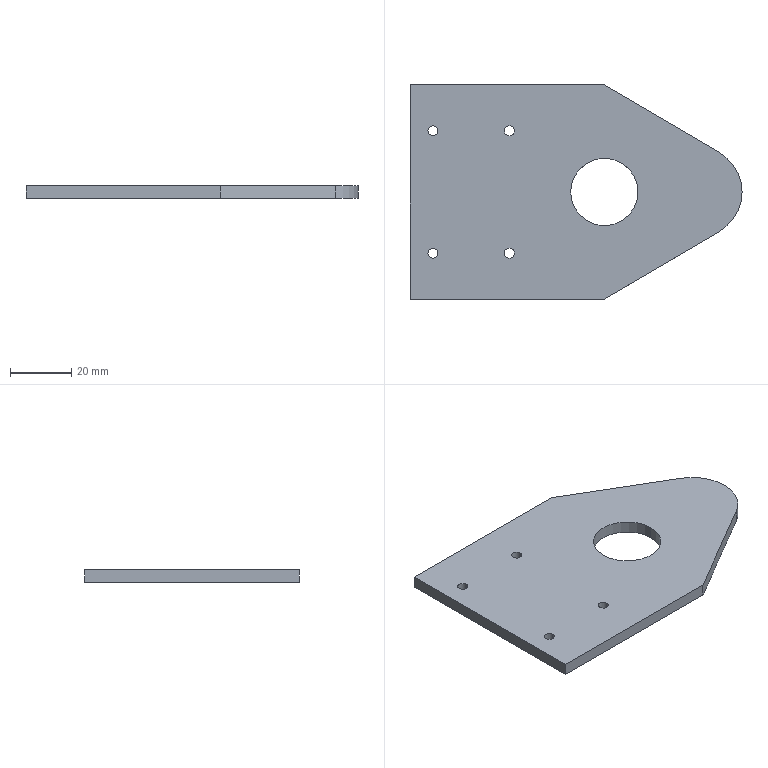Part | STEP file | Mounting plate | 1 solid | 19 faces | box 108.5 x 70 x 4 mm | volume 23874 mm3 | cylinder 12 | plane 7 | commonest cylinder face diameters 3.3 x8 22 x2 30 x2
STEP:
#1=CARTESIAN_POINT('',(-50.85,20.,-2.));
#2=VERTEX_POINT('',#1);
#3=CARTESIAN_POINT('',(-54.15,20.,-2.));
#4=VERTEX_POINT('',#3);
#5=CARTESIAN_POINT('',(-52.5,20.,-2.));
#6=DIRECTION('',(0.,0.,-1.));
#7=DIRECTION('',(-1.,0.,0.));
#8=AXIS2_PLACEMENT_3D('',#5,#6,#7);
#9=CIRCLE('',#8,1.65);
#10=EDGE_CURVE('',#2,#4,#9,.T.);
#11=ORIENTED_EDGE('',*,*,#10,.T.);
#12=CARTESIAN_POINT('',(-54.15,20.,2.));
#13=VERTEX_POINT('',#12);
#14=CARTESIAN_POINT('',(-54.15,20.,2.));
#15=DIRECTION('',(0.,0.,1.));
#16=VECTOR('',#15,1000.);
#17=LINE('',#14,#16);
#18=EDGE_CURVE('',#4,#13,#17,.T.);
#19=ORIENTED_EDGE('',*,*,#18,.T.);
#20=CARTESIAN_POINT('',(-50.85,20.,2.));
#21=VERTEX_POINT('',#20);
#22=CARTESIAN_POINT('',(-52.5,20.,2.));
#23=DIRECTION('',(0.,0.,1.));
#24=DIRECTION('',(1.,0.,0.));
#25=AXIS2_PLACEMENT_3D('',#22,#23,#24);
#26=CIRCLE('',#25,1.65);
#27=EDGE_CURVE('',#13,#21,#26,.T.);
#28=ORIENTED_EDGE('',*,*,#27,.T.);
#29=CARTESIAN_POINT('',(-50.85,20.,2.));
#30=DIRECTION('',(0.,0.,1.));
#31=VECTOR('',#30,1000.);
#32=LINE('',#29,#31);
#33=EDGE_CURVE('',#2,#21,#32,.T.);
#34=ORIENTED_EDGE('',*,*,#33,.F.);
#35=EDGE_LOOP('',(#11,#19,#28,#34));
#36=FACE_OUTER_BOUND('',#35,.T.);
#37=CARTESIAN_POINT('',(-52.5,20.,2.));
#38=DIRECTION('',(0.,0.,1.));
#39=DIRECTION('',(1.,0.,0.));
#40=AXIS2_PLACEMENT_3D('',#37,#38,#39);
#41=CYLINDRICAL_SURFACE('',#40,1.65);
#42=ADVANCED_FACE('',(#36),#41,.F.);
#43=CARTESIAN_POINT('',(-25.85,20.,-2.));
#44=VERTEX_POINT('',#43);
#45=CARTESIAN_POINT('',(-29.15,20.,-2.));
#46=VERTEX_POINT('',#45);
#47=CARTESIAN_POINT('',(-27.5,20.,-2.));
#48=DIRECTION('',(0.,0.,-1.));
#49=DIRECTION('',(-1.,0.,0.));
#50=AXIS2_PLACEMENT_3D('',#47,#48,#49);
#51=CIRCLE('',#50,1.65);
#52=EDGE_CURVE('',#44,#46,#51,.T.);
#53=ORIENTED_EDGE('',*,*,#52,.T.);
#54=CARTESIAN_POINT('',(-29.15,20.,2.));
#55=VERTEX_POINT('',#54);
#56=CARTESIAN_POINT('',(-29.15,20.,2.));
#57=DIRECTION('',(0.,0.,1.));
#58=VECTOR('',#57,1000.);
#59=LINE('',#56,#58);
#60=EDGE_CURVE('',#46,#55,#59,.T.);
#61=ORIENTED_EDGE('',*,*,#60,.T.);
#62=CARTESIAN_POINT('',(-25.85,20.,2.));
#63=VERTEX_POINT('',#62);
#64=CARTESIAN_POINT('',(-27.5,20.,2.));
#65=DIRECTION('',(0.,0.,1.));
#66=DIRECTION('',(1.,0.,0.));
#67=AXIS2_PLACEMENT_3D('',#64,#65,#66);
#68=CIRCLE('',#67,1.65);
#69=EDGE_CURVE('',#55,#63,#68,.T.);
#70=ORIENTED_EDGE('',*,*,#69,.T.);
#71=CARTESIAN_POINT('',(-25.85,20.,2.));
#72=DIRECTION('',(0.,0.,1.));
#73=VECTOR('',#72,1000.);
#74=LINE('',#71,#73);
#75=EDGE_CURVE('',#44,#63,#74,.T.);
#76=ORIENTED_EDGE('',*,*,#75,.F.);
#77=EDGE_LOOP('',(#53,#61,#70,#76));
#78=FACE_OUTER_BOUND('',#77,.T.);
#79=CARTESIAN_POINT('',(-27.5,20.,2.));
#80=DIRECTION('',(0.,0.,1.));
#81=DIRECTION('',(1.,0.,0.));
#82=AXIS2_PLACEMENT_3D('',#79,#80,#81);
#83=CYLINDRICAL_SURFACE('',#82,1.65);
#84=ADVANCED_FACE('',(#78),#83,.F.);
#85=CARTESIAN_POINT('',(-25.85,-20.,-2.));
#86=VERTEX_POINT('',#85);
#87=CARTESIAN_POINT('',(-29.15,-20.,-2.));
#88=VERTEX_POINT('',#87);
#89=CARTESIAN_POINT('',(-27.5,-20.,-2.));
#90=DIRECTION('',(0.,0.,-1.));
#91=DIRECTION('',(-1.,0.,0.));
#92=AXIS2_PLACEMENT_3D('',#89,#90,#91);
#93=CIRCLE('',#92,1.65);
#94=EDGE_CURVE('',#86,#88,#93,.T.);
#95=ORIENTED_EDGE('',*,*,#94,.T.);
#96=CARTESIAN_POINT('',(-29.15,-20.,2.));
#97=VERTEX_POINT('',#96);
#98=CARTESIAN_POINT('',(-29.15,-20.,2.));
#99=DIRECTION('',(0.,0.,1.));
#100=VECTOR('',#99,1000.);
#101=LINE('',#98,#100);
#102=EDGE_CURVE('',#88,#97,#101,.T.);
#103=ORIENTED_EDGE('',*,*,#102,.T.);
#104=CARTESIAN_POINT('',(-25.85,-20.,2.));
#105=VERTEX_POINT('',#104);
#106=CARTESIAN_POINT('',(-27.5,-20.,2.));
#107=DIRECTION('',(0.,0.,1.));
#108=DIRECTION('',(1.,0.,0.));
#109=AXIS2_PLACEMENT_3D('',#106,#107,#108);
#110=CIRCLE('',#109,1.65);
#111=EDGE_CURVE('',#97,#105,#110,.T.);
#112=ORIENTED_EDGE('',*,*,#111,.T.);
#113=CARTESIAN_POINT('',(-25.85,-20.,2.));
#114=DIRECTION('',(0.,0.,1.));
#115=VECTOR('',#114,1000.);
#116=LINE('',#113,#115);
#117=EDGE_CURVE('',#86,#105,#116,.T.);
#118=ORIENTED_EDGE('',*,*,#117,.F.);
#119=EDGE_LOOP('',(#95,#103,#112,#118));
#120=FACE_OUTER_BOUND('',#119,.T.);
#121=CARTESIAN_POINT('',(-27.5,-20.,2.));
#122=DIRECTION('',(0.,0.,1.));
#123=DIRECTION('',(1.,0.,0.));
#124=AXIS2_PLACEMENT_3D('',#121,#122,#123);
#125=CYLINDRICAL_SURFACE('',#124,1.65);
#126=ADVANCED_FACE('',(#120),#125,.F.);
#127=CARTESIAN_POINT('',(-50.85,-20.,-2.));
#128=VERTEX_POINT('',#127);
#129=CARTESIAN_POINT('',(-54.15,-20.,-2.));
#130=VERTEX_POINT('',#129);
#131=CARTESIAN_POINT('',(-52.5,-20.,-2.));
#132=DIRECTION('',(0.,0.,-1.));
#133=DIRECTION('',(-1.,0.,0.));
#134=AXIS2_PLACEMENT_3D('',#131,#132,#133);
#135=CIRCLE('',#134,1.65);
#136=EDGE_CURVE('',#128,#130,#135,.T.);
#137=ORIENTED_EDGE('',*,*,#136,.T.);
#138=CARTESIAN_POINT('',(-54.15,-20.,2.));
#139=VERTEX_POINT('',#138);
#140=CARTESIAN_POINT('',(-54.15,-20.,2.));
#141=DIRECTION('',(0.,0.,1.));
#142=VECTOR('',#141,1000.);
#143=LINE('',#140,#142);
#144=EDGE_CURVE('',#130,#139,#143,.T.);
#145=ORIENTED_EDGE('',*,*,#144,.T.);
#146=CARTESIAN_POINT('',(-50.85,-20.,2.));
#147=VERTEX_POINT('',#146);
#148=CARTESIAN_POINT('',(-52.5,-20.,2.));
#149=DIRECTION('',(0.,0.,1.));
#150=DIRECTION('',(1.,0.,0.));
#151=AXIS2_PLACEMENT_3D('',#148,#149,#150);
#152=CIRCLE('',#151,1.65);
#153=EDGE_CURVE('',#139,#147,#152,.T.);
#154=ORIENTED_EDGE('',*,*,#153,.T.);
#155=CARTESIAN_POINT('',(-50.85,-20.,2.));
#156=DIRECTION('',(0.,0.,1.));
#157=VECTOR('',#156,1000.);
#158=LINE('',#155,#157);
#159=EDGE_CURVE('',#128,#147,#158,.T.);
#160=ORIENTED_EDGE('',*,*,#159,.F.);
#161=EDGE_LOOP('',(#137,#145,#154,#160));
#162=FACE_OUTER_BOUND('',#161,.T.);
#163=CARTESIAN_POINT('',(-52.5,-20.,2.));
#164=DIRECTION('',(0.,0.,1.));
#165=DIRECTION('',(1.,0.,0.));
#166=AXIS2_PLACEMENT_3D('',#163,#164,#165);
#167=CYLINDRICAL_SURFACE('',#166,1.65);
#168=ADVANCED_FACE('',(#162),#167,.F.);
#169=CARTESIAN_POINT('',(48.5,0.,-2.));
#170=VERTEX_POINT('',#169);
#171=CARTESIAN_POINT('',(41.093,-12.936,-2.));
#172=VERTEX_POINT('',#171);
#173=CARTESIAN_POINT('',(33.5,0.,-2.));
#174=DIRECTION('',(0.,0.,-1.));
#175=DIRECTION('',(-1.,0.,0.));
#176=AXIS2_PLACEMENT_3D('',#173,#174,#175);
#177=CIRCLE('',#176,15.);
#178=EDGE_CURVE('',#170,#172,#177,.T.);
#179=ORIENTED_EDGE('',*,*,#178,.F.);
#180=CARTESIAN_POINT('',(48.5,0.,2.));
#181=VERTEX_POINT('',#180);
#182=CARTESIAN_POINT('',(48.5,0.,-2.001));
#183=DIRECTION('',(0.,0.,1.));
#184=VECTOR('',#183,1000.);
#185=LINE('',#182,#184);
#186=EDGE_CURVE('',#170,#181,#185,.T.);
#187=ORIENTED_EDGE('',*,*,#186,.T.);
#188=CARTESIAN_POINT('',(41.093,-12.936,2.));
#189=VERTEX_POINT('',#188);
#190=CARTESIAN_POINT('',(33.5,0.,2.));
#191=DIRECTION('',(0.,0.,-1.));
#192=DIRECTION('',(1.,0.,0.));
#193=AXIS2_PLACEMENT_3D('',#190,#191,#192);
#194=CIRCLE('',#193,15.);
#195=EDGE_CURVE('',#181,#189,#194,.T.);
#196=ORIENTED_EDGE('',*,*,#195,.T.);
#197=CARTESIAN_POINT('',(41.093,-12.936,-2.001));
#198=DIRECTION('',(0.,0.,1.));
#199=VECTOR('',#198,1000.);
#200=LINE('',#197,#199);
#201=EDGE_CURVE('',#172,#189,#200,.T.);
#202=ORIENTED_EDGE('',*,*,#201,.F.);
#203=EDGE_LOOP('',(#179,#187,#196,#202));
#204=FACE_OUTER_BOUND('',#203,.T.);
#205=CARTESIAN_POINT('',(33.5,0.,-2.001));
#206=DIRECTION('',(0.,0.,1.));
#207=DIRECTION('',(1.,0.,0.));
#208=AXIS2_PLACEMENT_3D('',#205,#206,#207);
#209=CYLINDRICAL_SURFACE('',#208,15.);
#210=ADVANCED_FACE('',(#204),#209,.T.);
#211=CARTESIAN_POINT('',(-7.5,0.,-2.));
#212=VERTEX_POINT('',#211);
#213=CARTESIAN_POINT('',(14.5,0.,-2.));
#214=VERTEX_POINT('',#213);
#215=CARTESIAN_POINT('',(3.5,0.,-2.));
#216=DIRECTION('',(0.,0.,1.));
#217=DIRECTION('',(-1.,0.,0.));
#218=AXIS2_PLACEMENT_3D('',#215,#216,#217);
#219=CIRCLE('',#218,11.);
#220=EDGE_CURVE('',#212,#214,#219,.T.);
#221=ORIENTED_EDGE('',*,*,#220,.F.);
#222=CARTESIAN_POINT('',(-7.5,0.,2.));
#223=VERTEX_POINT('',#222);
#224=CARTESIAN_POINT('',(-7.5,0.,-2.001));
#225=DIRECTION('',(0.,0.,1.));
#226=VECTOR('',#225,1000.);
#227=LINE('',#224,#226);
#228=EDGE_CURVE('',#212,#223,#227,.T.);
#229=ORIENTED_EDGE('',*,*,#228,.T.);
#230=CARTESIAN_POINT('',(14.5,0.,2.));
#231=VERTEX_POINT('',#230);
#232=CARTESIAN_POINT('',(3.5,0.,2.));
#233=DIRECTION('',(0.,0.,1.));
#234=DIRECTION('',(1.,0.,0.));
#235=AXIS2_PLACEMENT_3D('',#232,#233,#234);
#236=CIRCLE('',#235,11.);
#237=EDGE_CURVE('',#223,#231,#236,.T.);
#238=ORIENTED_EDGE('',*,*,#237,.T.);
#239=CARTESIAN_POINT('',(14.5,0.,-2.001));
#240=DIRECTION('',(0.,0.,1.));
#241=VECTOR('',#240,1000.);
#242=LINE('',#239,#241);
#243=EDGE_CURVE('',#214,#231,#242,.T.);
#244=ORIENTED_EDGE('',*,*,#243,.F.);
#245=EDGE_LOOP('',(#221,#229,#238,#244));
#246=FACE_OUTER_BOUND('',#245,.T.);
#247=CARTESIAN_POINT('',(3.5,0.,-2.001));
#248=DIRECTION('',(0.,0.,1.));
#249=DIRECTION('',(1.,0.,0.));
#250=AXIS2_PLACEMENT_3D('',#247,#248,#249);
#251=CYLINDRICAL_SURFACE('',#250,11.);
#252=ADVANCED_FACE('',(#246),#251,.F.);
#253=CARTESIAN_POINT('',(3.5,0.,2.));
#254=DIRECTION('',(0.,0.,1.));
#255=DIRECTION('',(1.,0.,0.));
#256=AXIS2_PLACEMENT_3D('',#253,#254,#255);
#257=CIRCLE('',#256,11.);
#258=EDGE_CURVE('',#231,#223,#257,.T.);
#259=ORIENTED_EDGE('',*,*,#258,.F.);
#260=ORIENTED_EDGE('',*,*,#237,.F.);
#261=EDGE_LOOP('',(#259,#260));
#262=FACE_BOUND('',#261,.T.);
#263=CARTESIAN_POINT('',(-60.,-35.,2.));
#264=VERTEX_POINT('',#263);
#265=CARTESIAN_POINT('',(3.5,-35.,2.));
#266=VERTEX_POINT('',#265);
#267=CARTESIAN_POINT('',(-60.,-35.,2.));
#268=DIRECTION('',(1.,0.,0.));
#269=VECTOR('',#268,1000.);
#270=LINE('',#267,#269);
#271=EDGE_CURVE('',#264,#266,#270,.T.);
#272=ORIENTED_EDGE('',*,*,#271,.T.);
#273=CARTESIAN_POINT('',(3.5,-35.,2.));
#274=DIRECTION('',(-0.8624,-0.5062,0.));
#275=VECTOR('',#274,1000.);
#276=LINE('',#273,#275);
#277=EDGE_CURVE('',#189,#266,#276,.T.);
#278=ORIENTED_EDGE('',*,*,#277,.F.);
#279=ORIENTED_EDGE('',*,*,#195,.F.);
#280=CARTESIAN_POINT('',(41.093,12.936,2.));
#281=VERTEX_POINT('',#280);
#282=CARTESIAN_POINT('',(33.5,0.,2.));
#283=DIRECTION('',(0.,0.,-1.));
#284=DIRECTION('',(1.,0.,0.));
#285=AXIS2_PLACEMENT_3D('',#282,#283,#284);
#286=CIRCLE('',#285,15.);
#287=EDGE_CURVE('',#281,#181,#286,.T.);
#288=ORIENTED_EDGE('',*,*,#287,.F.);
#289=CARTESIAN_POINT('',(3.5,35.,2.));
#290=VERTEX_POINT('',#289);
#291=CARTESIAN_POINT('',(3.5,35.,2.));
#292=DIRECTION('',(0.8624,-0.5062,0.));
#293=VECTOR('',#292,1000.);
#294=LINE('',#291,#293);
#295=EDGE_CURVE('',#290,#281,#294,.T.);
#296=ORIENTED_EDGE('',*,*,#295,.F.);
#297=CARTESIAN_POINT('',(-60.,35.,2.));
#298=VERTEX_POINT('',#297);
#299=CARTESIAN_POINT('',(-60.,35.,2.));
#300=DIRECTION('',(-1.,0.,0.));
#301=VECTOR('',#300,1000.);
#302=LINE('',#299,#301);
#303=EDGE_CURVE('',#290,#298,#302,.T.);
#304=ORIENTED_EDGE('',*,*,#303,.T.);
#305=CARTESIAN_POINT('',(-60.,-35.,2.));
#306=DIRECTION('',(0.,-1.,0.));
#307=VECTOR('',#306,1000.);
#308=LINE('',#305,#307);
#309=EDGE_CURVE('',#298,#264,#308,.T.);
#310=ORIENTED_EDGE('',*,*,#309,.T.);
#311=EDGE_LOOP('',(#272,#278,#279,#288,#296,#304,#310));
#312=FACE_OUTER_BOUND('',#311,.T.);
#313=CARTESIAN_POINT('',(-52.5,-20.,2.));
#314=DIRECTION('',(0.,0.,1.));
#315=DIRECTION('',(1.,0.,0.));
#316=AXIS2_PLACEMENT_3D('',#313,#314,#315);
#317=CIRCLE('',#316,1.65);
#318=EDGE_CURVE('',#147,#139,#317,.T.);
#319=ORIENTED_EDGE('',*,*,#318,.F.);
#320=ORIENTED_EDGE('',*,*,#153,.F.);
#321=EDGE_LOOP('',(#319,#320));
#322=FACE_BOUND('',#321,.T.);
#323=CARTESIAN_POINT('',(-27.5,-20.,2.));
#324=DIRECTION('',(0.,0.,1.));
#325=DIRECTION('',(1.,0.,0.));
#326=AXIS2_PLACEMENT_3D('',#323,#324,#325);
#327=CIRCLE('',#326,1.65);
#328=EDGE_CURVE('',#105,#97,#327,.T.);
#329=ORIENTED_EDGE('',*,*,#328,.F.);
#330=ORIENTED_EDGE('',*,*,#111,.F.);
#331=EDGE_LOOP('',(#329,#330));
#332=FACE_BOUND('',#331,.T.);
#333=CARTESIAN_POINT('',(-27.5,20.,2.));
#334=DIRECTION('',(0.,0.,1.));
#335=DIRECTION('',(1.,0.,0.));
#336=AXIS2_PLACEMENT_3D('',#333,#334,#335);
#337=CIRCLE('',#336,1.65);
#338=EDGE_CURVE('',#63,#55,#337,.T.);
#339=ORIENTED_EDGE('',*,*,#338,.F.);
#340=ORIENTED_EDGE('',*,*,#69,.F.);
#341=EDGE_LOOP('',(#339,#340));
#342=FACE_BOUND('',#341,.T.);
#343=CARTESIAN_POINT('',(-52.5,20.,2.));
#344=DIRECTION('',(0.,0.,1.));
#345=DIRECTION('',(1.,0.,0.));
#346=AXIS2_PLACEMENT_3D('',#343,#344,#345);
#347=CIRCLE('',#346,1.65);
#348=EDGE_CURVE('',#21,#13,#347,.T.);
#349=ORIENTED_EDGE('',*,*,#348,.F.);
#350=ORIENTED_EDGE('',*,*,#27,.F.);
#351=EDGE_LOOP('',(#349,#350));
#352=FACE_BOUND('',#351,.T.);
#353=CARTESIAN_POINT('',(0.,0.,2.));
#354=DIRECTION('',(0.,0.,-1.));
#355=DIRECTION('',(-1.,0.,0.));
#356=AXIS2_PLACEMENT_3D('',#353,#354,#355);
#357=PLANE('',#356);
#358=ADVANCED_FACE('',(#262,#312,#322,#332,#342,#352),#357,.F.);
#359=ORIENTED_EDGE('',*,*,#303,.F.);
#360=CARTESIAN_POINT('',(3.5,35.,-2.));
#361=VERTEX_POINT('',#360);
#362=CARTESIAN_POINT('',(3.5,35.,-2.001));
#363=DIRECTION('',(0.,0.,1.));
#364=VECTOR('',#363,1000.);
#365=LINE('',#362,#364);
#366=EDGE_CURVE('',#361,#290,#365,.T.);
#367=ORIENTED_EDGE('',*,*,#366,.F.);
#368=CARTESIAN_POINT('',(-60.,35.,-2.));
#369=VERTEX_POINT('',#368);
#370=CARTESIAN_POINT('',(-60.,35.,-2.));
#371=DIRECTION('',(-1.,0.,0.));
#372=VECTOR('',#371,1000.);
#373=LINE('',#370,#372);
#374=EDGE_CURVE('',#361,#369,#373,.T.);
#375=ORIENTED_EDGE('',*,*,#374,.T.);
#376=CARTESIAN_POINT('',(-60.,35.,2.));
#377=DIRECTION('',(0.,0.,-1.));
#378=VECTOR('',#377,1000.);
#379=LINE('',#376,#378);
#380=EDGE_CURVE('',#298,#369,#379,.T.);
#381=ORIENTED_EDGE('',*,*,#380,.F.);
#382=EDGE_LOOP('',(#359,#367,#375,#381));
#383=FACE_OUTER_BOUND('',#382,.T.);
#384=CARTESIAN_POINT('',(-60.,35.,2.));
#385=DIRECTION('',(0.,-1.,0.));
#386=DIRECTION('',(0.,0.,-1.));
#387=AXIS2_PLACEMENT_3D('',#384,#385,#386);
#388=PLANE('',#387);
#389=ADVANCED_FACE('',(#383),#388,.F.);
#390=CARTESIAN_POINT('',(-60.,-35.,-2.));
#391=VERTEX_POINT('',#390);
#392=CARTESIAN_POINT('',(-60.,-35.,-2.));
#393=DIRECTION('',(0.,-1.,0.));
#394=VECTOR('',#393,1000.);
#395=LINE('',#392,#394);
#396=EDGE_CURVE('',#369,#391,#395,.T.);
#397=ORIENTED_EDGE('',*,*,#396,.T.);
#398=CARTESIAN_POINT('',(-60.,-35.,2.));
#399=DIRECTION('',(0.,0.,-1.));
#400=VECTOR('',#399,1000.);
#401=LINE('',#398,#400);
#402=EDGE_CURVE('',#264,#391,#401,.T.);
#403=ORIENTED_EDGE('',*,*,#402,.F.);
#404=ORIENTED_EDGE('',*,*,#309,.F.);
#405=ORIENTED_EDGE('',*,*,#380,.T.);
#406=EDGE_LOOP('',(#397,#403,#404,#405));
#407=FACE_OUTER_BOUND('',#406,.T.);
#408=CARTESIAN_POINT('',(-60.,-35.,2.));
#409=DIRECTION('',(1.,0.,0.));
#410=DIRECTION('',(0.,0.,-1.));
#411=AXIS2_PLACEMENT_3D('',#408,#409,#410);
#412=PLANE('',#411);
#413=ADVANCED_FACE('',(#407),#412,.F.);
#414=CARTESIAN_POINT('',(3.5,-35.,-2.));
#415=VERTEX_POINT('',#414);
#416=CARTESIAN_POINT('',(-60.,-35.,-2.));
#417=DIRECTION('',(1.,0.,0.));
#418=VECTOR('',#417,1000.);
#419=LINE('',#416,#418);
#420=EDGE_CURVE('',#391,#415,#419,.T.);
#421=ORIENTED_EDGE('',*,*,#420,.T.);
#422=CARTESIAN_POINT('',(3.5,-35.,-2.001));
#423=DIRECTION('',(0.,0.,1.));
#424=VECTOR('',#423,1000.);
#425=LINE('',#422,#424);
#426=EDGE_CURVE('',#415,#266,#425,.T.);
#427=ORIENTED_EDGE('',*,*,#426,.T.);
#428=ORIENTED_EDGE('',*,*,#271,.F.);
#429=ORIENTED_EDGE('',*,*,#402,.T.);
#430=EDGE_LOOP('',(#421,#427,#428,#429));
#431=FACE_OUTER_BOUND('',#430,.T.);
#432=CARTESIAN_POINT('',(-60.,-35.,2.));
#433=DIRECTION('',(0.,1.,0.));
#434=DIRECTION('',(0.,0.,1.));
#435=AXIS2_PLACEMENT_3D('',#432,#433,#434);
#436=PLANE('',#435);
#437=ADVANCED_FACE('',(#431),#436,.F.);
#438=ORIENTED_EDGE('',*,*,#10,.F.);
#439=CARTESIAN_POINT('',(-52.5,20.,-2.));
#440=DIRECTION('',(0.,0.,-1.));
#441=DIRECTION('',(-1.,0.,0.));
#442=AXIS2_PLACEMENT_3D('',#439,#440,#441);
#443=CIRCLE('',#442,1.65);
#444=EDGE_CURVE('',#4,#2,#443,.T.);
#445=ORIENTED_EDGE('',*,*,#444,.F.);
#446=EDGE_LOOP('',(#438,#445));
#447=FACE_BOUND('',#446,.T.);
#448=ORIENTED_EDGE('',*,*,#52,.F.);
#449=CARTESIAN_POINT('',(-27.5,20.,-2.));
#450=DIRECTION('',(0.,0.,-1.));
#451=DIRECTION('',(-1.,0.,0.));
#452=AXIS2_PLACEMENT_3D('',#449,#450,#451);
#453=CIRCLE('',#452,1.65);
#454=EDGE_CURVE('',#46,#44,#453,.T.);
#455=ORIENTED_EDGE('',*,*,#454,.F.);
#456=EDGE_LOOP('',(#448,#455));
#457=FACE_BOUND('',#456,.T.);
#458=ORIENTED_EDGE('',*,*,#94,.F.);
#459=CARTESIAN_POINT('',(-27.5,-20.,-2.));
#460=DIRECTION('',(0.,0.,-1.));
#461=DIRECTION('',(-1.,0.,0.));
#462=AXIS2_PLACEMENT_3D('',#459,#460,#461);
#463=CIRCLE('',#462,1.65);
#464=EDGE_CURVE('',#88,#86,#463,.T.);
#465=ORIENTED_EDGE('',*,*,#464,.F.);
#466=EDGE_LOOP('',(#458,#465));
#467=FACE_BOUND('',#466,.T.);
#468=ORIENTED_EDGE('',*,*,#136,.F.);
#469=CARTESIAN_POINT('',(-52.5,-20.,-2.));
#470=DIRECTION('',(0.,0.,-1.));
#471=DIRECTION('',(-1.,0.,0.));
#472=AXIS2_PLACEMENT_3D('',#469,#470,#471);
#473=CIRCLE('',#472,1.65);
#474=EDGE_CURVE('',#130,#128,#473,.T.);
#475=ORIENTED_EDGE('',*,*,#474,.F.);
#476=EDGE_LOOP('',(#468,#475));
#477=FACE_BOUND('',#476,.T.);
#478=CARTESIAN_POINT('',(3.5,-35.,-2.));
#479=DIRECTION('',(-0.8624,-0.5062,0.));
#480=VECTOR('',#479,1000.);
#481=LINE('',#478,#480);
#482=EDGE_CURVE('',#172,#415,#481,.T.);
#483=ORIENTED_EDGE('',*,*,#482,.T.);
#484=ORIENTED_EDGE('',*,*,#420,.F.);
#485=ORIENTED_EDGE('',*,*,#396,.F.);
#486=ORIENTED_EDGE('',*,*,#374,.F.);
#487=CARTESIAN_POINT('',(41.093,12.936,-2.));
#488=VERTEX_POINT('',#487);
#489=CARTESIAN_POINT('',(3.5,35.,-2.));
#490=DIRECTION('',(0.8624,-0.5062,0.));
#491=VECTOR('',#490,1000.);
#492=LINE('',#489,#491);
#493=EDGE_CURVE('',#361,#488,#492,.T.);
#494=ORIENTED_EDGE('',*,*,#493,.T.);
#495=CARTESIAN_POINT('',(33.5,0.,-2.));
#496=DIRECTION('',(0.,0.,-1.));
#497=DIRECTION('',(-1.,0.,0.));
#498=AXIS2_PLACEMENT_3D('',#495,#496,#497);
#499=CIRCLE('',#498,15.);
#500=EDGE_CURVE('',#488,#170,#499,.T.);
#501=ORIENTED_EDGE('',*,*,#500,.T.);
#502=ORIENTED_EDGE('',*,*,#178,.T.);
#503=EDGE_LOOP('',(#483,#484,#485,#486,#494,#501,#502));
#504=FACE_OUTER_BOUND('',#503,.T.);
#505=CARTESIAN_POINT('',(3.5,0.,-2.));
#506=DIRECTION('',(0.,0.,1.));
#507=DIRECTION('',(-1.,0.,0.));
#508=AXIS2_PLACEMENT_3D('',#505,#506,#507);
#509=CIRCLE('',#508,11.);
#510=EDGE_CURVE('',#214,#212,#509,.T.);
#511=ORIENTED_EDGE('',*,*,#510,.T.);
#512=ORIENTED_EDGE('',*,*,#220,.T.);
#513=EDGE_LOOP('',(#511,#512));
#514=FACE_BOUND('',#513,.T.);
#515=CARTESIAN_POINT('',(0.,0.,-2.));
#516=DIRECTION('',(0.,0.,-1.));
#517=DIRECTION('',(-1.,0.,0.));
#518=AXIS2_PLACEMENT_3D('',#515,#516,#517);
#519=PLANE('',#518);
#520=ADVANCED_FACE('',(#447,#457,#467,#477,#504,#514),#519,.T.);
#521=ORIENTED_EDGE('',*,*,#228,.F.);
#522=ORIENTED_EDGE('',*,*,#510,.F.);
#523=ORIENTED_EDGE('',*,*,#243,.T.);
#524=ORIENTED_EDGE('',*,*,#258,.T.);
#525=EDGE_LOOP('',(#521,#522,#523,#524));
#526=FACE_OUTER_BOUND('',#525,.T.);
#527=CARTESIAN_POINT('',(3.5,0.,-2.001));
#528=DIRECTION('',(0.,0.,1.));
#529=DIRECTION('',(1.,0.,0.));
#530=AXIS2_PLACEMENT_3D('',#527,#528,#529);
#531=CYLINDRICAL_SURFACE('',#530,11.);
#532=ADVANCED_FACE('',(#526),#531,.F.);
#533=ORIENTED_EDGE('',*,*,#201,.T.);
#534=ORIENTED_EDGE('',*,*,#277,.T.);
#535=ORIENTED_EDGE('',*,*,#426,.F.);
#536=ORIENTED_EDGE('',*,*,#482,.F.);
#537=EDGE_LOOP('',(#533,#534,#535,#536));
#538=FACE_OUTER_BOUND('',#537,.T.);
#539=CARTESIAN_POINT('',(3.5,-35.,-2.001));
#540=DIRECTION('',(-0.5062,0.8624,0.));
#541=DIRECTION('',(-0.8624,-0.5062,0.));
#542=AXIS2_PLACEMENT_3D('',#539,#540,#541);
#543=PLANE('',#542);
#544=ADVANCED_FACE('',(#538),#543,.F.);
#545=ORIENTED_EDGE('',*,*,#186,.F.);
#546=ORIENTED_EDGE('',*,*,#500,.F.);
#547=CARTESIAN_POINT('',(41.093,12.936,-2.001));
#548=DIRECTION('',(0.,0.,1.));
#549=VECTOR('',#548,1000.);
#550=LINE('',#547,#549);
#551=EDGE_CURVE('',#488,#281,#550,.T.);
#552=ORIENTED_EDGE('',*,*,#551,.T.);
#553=ORIENTED_EDGE('',*,*,#287,.T.);
#554=EDGE_LOOP('',(#545,#546,#552,#553));
#555=FACE_OUTER_BOUND('',#554,.T.);
#556=CARTESIAN_POINT('',(33.5,0.,-2.001));
#557=DIRECTION('',(0.,0.,1.));
#558=DIRECTION('',(1.,0.,0.));
#559=AXIS2_PLACEMENT_3D('',#556,#557,#558);
#560=CYLINDRICAL_SURFACE('',#559,15.);
#561=ADVANCED_FACE('',(#555),#560,.T.);
#562=ORIENTED_EDGE('',*,*,#366,.T.);
#563=ORIENTED_EDGE('',*,*,#295,.T.);
#564=ORIENTED_EDGE('',*,*,#551,.F.);
#565=ORIENTED_EDGE('',*,*,#493,.F.);
#566=EDGE_LOOP('',(#562,#563,#564,#565));
#567=FACE_OUTER_BOUND('',#566,.T.);
#568=CARTESIAN_POINT('',(3.5,35.,-2.001));
#569=DIRECTION('',(-0.5062,-0.8624,0.));
#570=DIRECTION('',(0.8624,-0.5062,0.));
#571=AXIS2_PLACEMENT_3D('',#568,#569,#570);
#572=PLANE('',#571);
#573=ADVANCED_FACE('',(#567),#572,.F.);
#574=ORIENTED_EDGE('',*,*,#144,.F.);
#575=ORIENTED_EDGE('',*,*,#474,.T.);
#576=ORIENTED_EDGE('',*,*,#159,.T.);
#577=ORIENTED_EDGE('',*,*,#318,.T.);
#578=EDGE_LOOP('',(#574,#575,#576,#577));
#579=FACE_OUTER_BOUND('',#578,.T.);
#580=CARTESIAN_POINT('',(-52.5,-20.,2.));
#581=DIRECTION('',(0.,0.,1.));
#582=DIRECTION('',(1.,0.,0.));
#583=AXIS2_PLACEMENT_3D('',#580,#581,#582);
#584=CYLINDRICAL_SURFACE('',#583,1.65);
#585=ADVANCED_FACE('',(#579),#584,.F.);
#586=ORIENTED_EDGE('',*,*,#102,.F.);
#587=ORIENTED_EDGE('',*,*,#464,.T.);
#588=ORIENTED_EDGE('',*,*,#117,.T.);
#589=ORIENTED_EDGE('',*,*,#328,.T.);
#590=EDGE_LOOP('',(#586,#587,#588,#589));
#591=FACE_OUTER_BOUND('',#590,.T.);
#592=CARTESIAN_POINT('',(-27.5,-20.,2.));
#593=DIRECTION('',(0.,0.,1.));
#594=DIRECTION('',(1.,0.,0.));
#595=AXIS2_PLACEMENT_3D('',#592,#593,#594);
#596=CYLINDRICAL_SURFACE('',#595,1.65);
#597=ADVANCED_FACE('',(#591),#596,.F.);
#598=ORIENTED_EDGE('',*,*,#60,.F.);
#599=ORIENTED_EDGE('',*,*,#454,.T.);
#600=ORIENTED_EDGE('',*,*,#75,.T.);
#601=ORIENTED_EDGE('',*,*,#338,.T.);
#602=EDGE_LOOP('',(#598,#599,#600,#601));
#603=FACE_OUTER_BOUND('',#602,.T.);
#604=CARTESIAN_POINT('',(-27.5,20.,2.));
#605=DIRECTION('',(0.,0.,1.));
#606=DIRECTION('',(1.,0.,0.));
#607=AXIS2_PLACEMENT_3D('',#604,#605,#606);
#608=CYLINDRICAL_SURFACE('',#607,1.65);
#609=ADVANCED_FACE('',(#603),#608,.F.);
#610=ORIENTED_EDGE('',*,*,#18,.F.);
#611=ORIENTED_EDGE('',*,*,#444,.T.);
#612=ORIENTED_EDGE('',*,*,#33,.T.);
#613=ORIENTED_EDGE('',*,*,#348,.T.);
#614=EDGE_LOOP('',(#610,#611,#612,#613));
#615=FACE_OUTER_BOUND('',#614,.T.);
#616=CARTESIAN_POINT('',(-52.5,20.,2.));
#617=DIRECTION('',(0.,0.,1.));
#618=DIRECTION('',(1.,0.,0.));
#619=AXIS2_PLACEMENT_3D('',#616,#617,#618);
#620=CYLINDRICAL_SURFACE('',#619,1.65);
#621=ADVANCED_FACE('',(#615),#620,.F.);
#622=CLOSED_SHELL('',(#42,#84,#126,#168,#210,#252,#358,#389,#413,#437,#520,#532,#544,#561,#573,#585,#597,#609,#621));
#623=MANIFOLD_SOLID_BREP('',#622);
#624=CARTESIAN_POINT('',(0.,0.,0.));
#625=DIRECTION('',(0.,0.,1.));
#626=DIRECTION('',(1.,0.,0.));
#627=AXIS2_PLACEMENT_3D('',#624,#625,#626);
#628=(LENGTH_UNIT()NAMED_UNIT(*)SI_UNIT(.MILLI.,.METRE.));
#629=UNCERTAINTY_MEASURE_WITH_UNIT(LENGTH_MEASURE(0.00001),#628,'','');
#630=(NAMED_UNIT(*)PLANE_ANGLE_UNIT()SI_UNIT($,.RADIAN.));
#631=(NAMED_UNIT(*)SI_UNIT($,.STERADIAN.)SOLID_ANGLE_UNIT());
#632=(GEOMETRIC_REPRESENTATION_CONTEXT(3)GLOBAL_UNCERTAINTY_ASSIGNED_CONTEXT((#629))GLOBAL_UNIT_ASSIGNED_CONTEXT((#628,#630,#631))REPRESENTATION_CONTEXT('',''));
#633=ADVANCED_BREP_SHAPE_REPRESENTATION('',(#623,#627),#632);